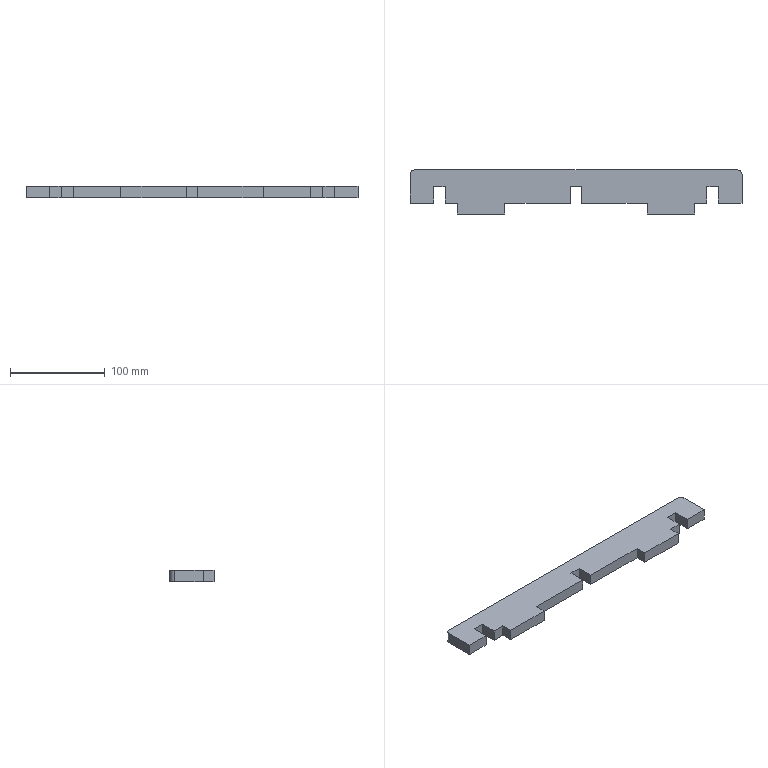Part | SolidWorks | features FlatPattern 1, SMBaseFlange 1, SheetMetal 1 | 1 solid | 28 faces | box 350 x 46.5 x 12 mm | volume 153111 mm3 | plane 26 | cylinder 2 | commonest cylinder face diameters 10 x2
STEP:
#1=CARTESIAN_POINT('',(187.743,-232.937,0.));
#2=VERTEX_POINT('',#1);
#3=CARTESIAN_POINT('',(187.743,-202.937,0.));
#4=VERTEX_POINT('',#3);
#5=CARTESIAN_POINT('',(187.743,-202.937,0.));
#6=DIRECTION('',(0.,1.,0.));
#7=VECTOR('',#6,1000.);
#8=LINE('',#5,#7);
#9=EDGE_CURVE('',#2,#4,#8,.T.);
#10=ORIENTED_EDGE('',*,*,#9,.F.);
#11=CARTESIAN_POINT('',(187.743,-232.937,-12.));
#12=VERTEX_POINT('',#11);
#13=CARTESIAN_POINT('',(187.743,-232.937,-12.));
#14=DIRECTION('',(0.,0.,1.));
#15=VECTOR('',#14,1000.);
#16=LINE('',#13,#15);
#17=EDGE_CURVE('',#12,#2,#16,.T.);
#18=ORIENTED_EDGE('',*,*,#17,.F.);
#19=CARTESIAN_POINT('',(187.743,-202.937,-12.));
#20=VERTEX_POINT('',#19);
#21=CARTESIAN_POINT('',(187.743,-202.937,-12.));
#22=DIRECTION('',(0.,1.,0.));
#23=VECTOR('',#22,1000.);
#24=LINE('',#21,#23);
#25=EDGE_CURVE('',#12,#20,#24,.T.);
#26=ORIENTED_EDGE('',*,*,#25,.T.);
#27=CARTESIAN_POINT('',(187.743,-202.937,-12.));
#28=DIRECTION('',(0.,0.,1.));
#29=VECTOR('',#28,1000.);
#30=LINE('',#27,#29);
#31=EDGE_CURVE('',#20,#4,#30,.T.);
#32=ORIENTED_EDGE('',*,*,#31,.T.);
#33=EDGE_LOOP('',(#10,#18,#26,#32));
#34=FACE_OUTER_BOUND('',#33,.T.);
#35=CARTESIAN_POINT('',(187.743,-202.937,-12.));
#36=DIRECTION('',(1.,0.,0.));
#37=DIRECTION('',(0.,0.,-1.));
#38=AXIS2_PLACEMENT_3D('',#35,#36,#37);
#39=PLANE('',#38);
#40=ADVANCED_FACE('',(#34),#39,.T.);
#41=CARTESIAN_POINT('',(162.743,-232.937,0.));
#42=VERTEX_POINT('',#41);
#43=CARTESIAN_POINT('',(187.743,-232.937,0.));
#44=DIRECTION('',(1.,0.,0.));
#45=VECTOR('',#44,1000.);
#46=LINE('',#43,#45);
#47=EDGE_CURVE('',#42,#2,#46,.T.);
#48=ORIENTED_EDGE('',*,*,#47,.F.);
#49=CARTESIAN_POINT('',(162.743,-232.937,-12.));
#50=VERTEX_POINT('',#49);
#51=CARTESIAN_POINT('',(162.743,-232.937,-12.));
#52=DIRECTION('',(0.,0.,1.));
#53=VECTOR('',#52,1000.);
#54=LINE('',#51,#53);
#55=EDGE_CURVE('',#50,#42,#54,.T.);
#56=ORIENTED_EDGE('',*,*,#55,.F.);
#57=CARTESIAN_POINT('',(187.743,-232.937,-12.));
#58=DIRECTION('',(1.,0.,0.));
#59=VECTOR('',#58,1000.);
#60=LINE('',#57,#59);
#61=EDGE_CURVE('',#50,#12,#60,.T.);
#62=ORIENTED_EDGE('',*,*,#61,.T.);
#63=ORIENTED_EDGE('',*,*,#17,.T.);
#64=EDGE_LOOP('',(#48,#56,#62,#63));
#65=FACE_OUTER_BOUND('',#64,.T.);
#66=CARTESIAN_POINT('',(187.743,-232.937,-12.));
#67=DIRECTION('',(0.,-1.,0.));
#68=DIRECTION('',(0.,0.,-1.));
#69=AXIS2_PLACEMENT_3D('',#66,#67,#68);
#70=PLANE('',#69);
#71=ADVANCED_FACE('',(#65),#70,.T.);
#72=CARTESIAN_POINT('',(162.743,-215.437,0.));
#73=VERTEX_POINT('',#72);
#74=CARTESIAN_POINT('',(162.743,-232.937,0.));
#75=DIRECTION('',(0.,-1.,0.));
#76=VECTOR('',#75,1000.);
#77=LINE('',#74,#76);
#78=EDGE_CURVE('',#73,#42,#77,.T.);
#79=ORIENTED_EDGE('',*,*,#78,.F.);
#80=CARTESIAN_POINT('',(162.743,-215.437,-12.));
#81=VERTEX_POINT('',#80);
#82=CARTESIAN_POINT('',(162.743,-215.437,-12.));
#83=DIRECTION('',(0.,0.,1.));
#84=VECTOR('',#83,1000.);
#85=LINE('',#82,#84);
#86=EDGE_CURVE('',#81,#73,#85,.T.);
#87=ORIENTED_EDGE('',*,*,#86,.F.);
#88=CARTESIAN_POINT('',(162.743,-232.937,-12.));
#89=DIRECTION('',(0.,-1.,0.));
#90=VECTOR('',#89,1000.);
#91=LINE('',#88,#90);
#92=EDGE_CURVE('',#81,#50,#91,.T.);
#93=ORIENTED_EDGE('',*,*,#92,.T.);
#94=ORIENTED_EDGE('',*,*,#55,.T.);
#95=EDGE_LOOP('',(#79,#87,#93,#94));
#96=FACE_OUTER_BOUND('',#95,.T.);
#97=CARTESIAN_POINT('',(162.743,-232.937,-12.));
#98=DIRECTION('',(-1.,0.,0.));
#99=DIRECTION('',(0.,-1.,0.));
#100=AXIS2_PLACEMENT_3D('',#97,#98,#99);
#101=PLANE('',#100);
#102=ADVANCED_FACE('',(#96),#101,.T.);
#103=CARTESIAN_POINT('',(150.743,-215.437,0.));
#104=VERTEX_POINT('',#103);
#105=CARTESIAN_POINT('',(162.743,-215.437,0.));
#106=DIRECTION('',(1.,0.,0.));
#107=VECTOR('',#106,1000.);
#108=LINE('',#105,#107);
#109=EDGE_CURVE('',#104,#73,#108,.T.);
#110=ORIENTED_EDGE('',*,*,#109,.F.);
#111=CARTESIAN_POINT('',(150.743,-215.437,-12.));
#112=VERTEX_POINT('',#111);
#113=CARTESIAN_POINT('',(150.743,-215.437,-12.));
#114=DIRECTION('',(0.,0.,1.));
#115=VECTOR('',#114,1000.);
#116=LINE('',#113,#115);
#117=EDGE_CURVE('',#112,#104,#116,.T.);
#118=ORIENTED_EDGE('',*,*,#117,.F.);
#119=CARTESIAN_POINT('',(162.743,-215.437,-12.));
#120=DIRECTION('',(1.,0.,0.));
#121=VECTOR('',#120,1000.);
#122=LINE('',#119,#121);
#123=EDGE_CURVE('',#112,#81,#122,.T.);
#124=ORIENTED_EDGE('',*,*,#123,.T.);
#125=ORIENTED_EDGE('',*,*,#86,.T.);
#126=EDGE_LOOP('',(#110,#118,#124,#125));
#127=FACE_OUTER_BOUND('',#126,.T.);
#128=CARTESIAN_POINT('',(162.743,-215.437,-12.));
#129=DIRECTION('',(0.,-1.,0.));
#130=DIRECTION('',(0.,0.,-1.));
#131=AXIS2_PLACEMENT_3D('',#128,#129,#130);
#132=PLANE('',#131);
#133=ADVANCED_FACE('',(#127),#132,.T.);
#134=CARTESIAN_POINT('',(150.743,-232.937,0.));
#135=VERTEX_POINT('',#134);
#136=CARTESIAN_POINT('',(150.743,-215.437,0.));
#137=DIRECTION('',(0.,1.,0.));
#138=VECTOR('',#137,1000.);
#139=LINE('',#136,#138);
#140=EDGE_CURVE('',#135,#104,#139,.T.);
#141=ORIENTED_EDGE('',*,*,#140,.F.);
#142=CARTESIAN_POINT('',(150.743,-232.937,-12.));
#143=VERTEX_POINT('',#142);
#144=CARTESIAN_POINT('',(150.743,-232.937,-12.));
#145=DIRECTION('',(0.,0.,1.));
#146=VECTOR('',#145,1000.);
#147=LINE('',#144,#146);
#148=EDGE_CURVE('',#143,#135,#147,.T.);
#149=ORIENTED_EDGE('',*,*,#148,.F.);
#150=CARTESIAN_POINT('',(150.743,-215.437,-12.));
#151=DIRECTION('',(0.,1.,0.));
#152=VECTOR('',#151,1000.);
#153=LINE('',#150,#152);
#154=EDGE_CURVE('',#143,#112,#153,.T.);
#155=ORIENTED_EDGE('',*,*,#154,.T.);
#156=ORIENTED_EDGE('',*,*,#117,.T.);
#157=EDGE_LOOP('',(#141,#149,#155,#156));
#158=FACE_OUTER_BOUND('',#157,.T.);
#159=CARTESIAN_POINT('',(150.743,-215.437,-12.));
#160=DIRECTION('',(1.,0.,0.));
#161=DIRECTION('',(0.,0.,-1.));
#162=AXIS2_PLACEMENT_3D('',#159,#160,#161);
#163=PLANE('',#162);
#164=ADVANCED_FACE('',(#158),#163,.T.);
#165=CARTESIAN_POINT('',(137.743,-232.937,0.));
#166=VERTEX_POINT('',#165);
#167=CARTESIAN_POINT('',(150.743,-232.937,0.));
#168=DIRECTION('',(1.,0.,0.));
#169=VECTOR('',#168,1000.);
#170=LINE('',#167,#169);
#171=EDGE_CURVE('',#166,#135,#170,.T.);
#172=ORIENTED_EDGE('',*,*,#171,.F.);
#173=CARTESIAN_POINT('',(137.743,-232.937,-12.));
#174=VERTEX_POINT('',#173);
#175=CARTESIAN_POINT('',(137.743,-232.937,-12.));
#176=DIRECTION('',(0.,0.,1.));
#177=VECTOR('',#176,1000.);
#178=LINE('',#175,#177);
#179=EDGE_CURVE('',#174,#166,#178,.T.);
#180=ORIENTED_EDGE('',*,*,#179,.F.);
#181=CARTESIAN_POINT('',(150.743,-232.937,-12.));
#182=DIRECTION('',(1.,0.,0.));
#183=VECTOR('',#182,1000.);
#184=LINE('',#181,#183);
#185=EDGE_CURVE('',#174,#143,#184,.T.);
#186=ORIENTED_EDGE('',*,*,#185,.T.);
#187=ORIENTED_EDGE('',*,*,#148,.T.);
#188=EDGE_LOOP('',(#172,#180,#186,#187));
#189=FACE_OUTER_BOUND('',#188,.T.);
#190=CARTESIAN_POINT('',(150.743,-232.937,-12.));
#191=DIRECTION('',(0.,-1.,0.));
#192=DIRECTION('',(0.,0.,-1.));
#193=AXIS2_PLACEMENT_3D('',#190,#191,#192);
#194=PLANE('',#193);
#195=ADVANCED_FACE('',(#189),#194,.T.);
#196=CARTESIAN_POINT('',(137.743,-244.437,0.));
#197=VERTEX_POINT('',#196);
#198=CARTESIAN_POINT('',(137.743,-232.937,0.));
#199=DIRECTION('',(0.,1.,0.));
#200=VECTOR('',#199,1000.);
#201=LINE('',#198,#200);
#202=EDGE_CURVE('',#197,#166,#201,.T.);
#203=ORIENTED_EDGE('',*,*,#202,.F.);
#204=CARTESIAN_POINT('',(137.743,-244.437,-12.));
#205=VERTEX_POINT('',#204);
#206=CARTESIAN_POINT('',(137.743,-244.437,-12.));
#207=DIRECTION('',(0.,0.,1.));
#208=VECTOR('',#207,1000.);
#209=LINE('',#206,#208);
#210=EDGE_CURVE('',#205,#197,#209,.T.);
#211=ORIENTED_EDGE('',*,*,#210,.F.);
#212=CARTESIAN_POINT('',(137.743,-232.937,-12.));
#213=DIRECTION('',(0.,1.,0.));
#214=VECTOR('',#213,1000.);
#215=LINE('',#212,#214);
#216=EDGE_CURVE('',#205,#174,#215,.T.);
#217=ORIENTED_EDGE('',*,*,#216,.T.);
#218=ORIENTED_EDGE('',*,*,#179,.T.);
#219=EDGE_LOOP('',(#203,#211,#217,#218));
#220=FACE_OUTER_BOUND('',#219,.T.);
#221=CARTESIAN_POINT('',(137.743,-232.937,-12.));
#222=DIRECTION('',(1.,0.,0.));
#223=DIRECTION('',(0.,0.,-1.));
#224=AXIS2_PLACEMENT_3D('',#221,#222,#223);
#225=PLANE('',#224);
#226=ADVANCED_FACE('',(#220),#225,.T.);
#227=CARTESIAN_POINT('',(87.743,-244.437,0.));
#228=VERTEX_POINT('',#227);
#229=CARTESIAN_POINT('',(137.743,-244.437,0.));
#230=DIRECTION('',(1.,0.,0.));
#231=VECTOR('',#230,1000.);
#232=LINE('',#229,#231);
#233=EDGE_CURVE('',#228,#197,#232,.T.);
#234=ORIENTED_EDGE('',*,*,#233,.F.);
#235=CARTESIAN_POINT('',(87.743,-244.437,-12.));
#236=VERTEX_POINT('',#235);
#237=CARTESIAN_POINT('',(87.743,-244.437,-12.));
#238=DIRECTION('',(0.,0.,1.));
#239=VECTOR('',#238,1000.);
#240=LINE('',#237,#239);
#241=EDGE_CURVE('',#236,#228,#240,.T.);
#242=ORIENTED_EDGE('',*,*,#241,.F.);
#243=CARTESIAN_POINT('',(137.743,-244.437,-12.));
#244=DIRECTION('',(1.,0.,0.));
#245=VECTOR('',#244,1000.);
#246=LINE('',#243,#245);
#247=EDGE_CURVE('',#236,#205,#246,.T.);
#248=ORIENTED_EDGE('',*,*,#247,.T.);
#249=ORIENTED_EDGE('',*,*,#210,.T.);
#250=EDGE_LOOP('',(#234,#242,#248,#249));
#251=FACE_OUTER_BOUND('',#250,.T.);
#252=CARTESIAN_POINT('',(137.743,-244.437,-12.));
#253=DIRECTION('',(0.,-1.,0.));
#254=DIRECTION('',(0.,0.,-1.));
#255=AXIS2_PLACEMENT_3D('',#252,#253,#254);
#256=PLANE('',#255);
#257=ADVANCED_FACE('',(#251),#256,.T.);
#258=CARTESIAN_POINT('',(87.743,-232.937,0.));
#259=VERTEX_POINT('',#258);
#260=CARTESIAN_POINT('',(87.743,-244.437,0.));
#261=DIRECTION('',(0.,-1.,0.));
#262=VECTOR('',#261,1000.);
#263=LINE('',#260,#262);
#264=EDGE_CURVE('',#259,#228,#263,.T.);
#265=ORIENTED_EDGE('',*,*,#264,.F.);
#266=CARTESIAN_POINT('',(87.743,-232.937,-12.));
#267=VERTEX_POINT('',#266);
#268=CARTESIAN_POINT('',(87.743,-232.937,-12.));
#269=DIRECTION('',(0.,0.,1.));
#270=VECTOR('',#269,1000.);
#271=LINE('',#268,#270);
#272=EDGE_CURVE('',#267,#259,#271,.T.);
#273=ORIENTED_EDGE('',*,*,#272,.F.);
#274=CARTESIAN_POINT('',(87.743,-244.437,-12.));
#275=DIRECTION('',(0.,-1.,0.));
#276=VECTOR('',#275,1000.);
#277=LINE('',#274,#276);
#278=EDGE_CURVE('',#267,#236,#277,.T.);
#279=ORIENTED_EDGE('',*,*,#278,.T.);
#280=ORIENTED_EDGE('',*,*,#241,.T.);
#281=EDGE_LOOP('',(#265,#273,#279,#280));
#282=FACE_OUTER_BOUND('',#281,.T.);
#283=CARTESIAN_POINT('',(87.743,-244.437,-12.));
#284=DIRECTION('',(-1.,0.,0.));
#285=DIRECTION('',(0.,0.,1.));
#286=AXIS2_PLACEMENT_3D('',#283,#284,#285);
#287=PLANE('',#286);
#288=ADVANCED_FACE('',(#282),#287,.T.);
#289=CARTESIAN_POINT('',(18.743,-232.937,0.));
#290=VERTEX_POINT('',#289);
#291=CARTESIAN_POINT('',(87.743,-232.937,0.));
#292=DIRECTION('',(1.,0.,0.));
#293=VECTOR('',#292,1000.);
#294=LINE('',#291,#293);
#295=EDGE_CURVE('',#290,#259,#294,.T.);
#296=ORIENTED_EDGE('',*,*,#295,.F.);
#297=CARTESIAN_POINT('',(18.743,-232.937,-12.));
#298=VERTEX_POINT('',#297);
#299=CARTESIAN_POINT('',(18.743,-232.937,-12.));
#300=DIRECTION('',(0.,0.,1.));
#301=VECTOR('',#300,1000.);
#302=LINE('',#299,#301);
#303=EDGE_CURVE('',#298,#290,#302,.T.);
#304=ORIENTED_EDGE('',*,*,#303,.F.);
#305=CARTESIAN_POINT('',(87.743,-232.937,-12.));
#306=DIRECTION('',(1.,0.,0.));
#307=VECTOR('',#306,1000.);
#308=LINE('',#305,#307);
#309=EDGE_CURVE('',#298,#267,#308,.T.);
#310=ORIENTED_EDGE('',*,*,#309,.T.);
#311=ORIENTED_EDGE('',*,*,#272,.T.);
#312=EDGE_LOOP('',(#296,#304,#310,#311));
#313=FACE_OUTER_BOUND('',#312,.T.);
#314=CARTESIAN_POINT('',(87.743,-232.937,-12.));
#315=DIRECTION('',(0.,-1.,0.));
#316=DIRECTION('',(1.,0.,0.));
#317=AXIS2_PLACEMENT_3D('',#314,#315,#316);
#318=PLANE('',#317);
#319=ADVANCED_FACE('',(#313),#318,.T.);
#320=CARTESIAN_POINT('',(18.743,-215.437,0.));
#321=VERTEX_POINT('',#320);
#322=CARTESIAN_POINT('',(18.743,-232.937,0.));
#323=DIRECTION('',(0.,-1.,0.));
#324=VECTOR('',#323,1000.);
#325=LINE('',#322,#324);
#326=EDGE_CURVE('',#321,#290,#325,.T.);
#327=ORIENTED_EDGE('',*,*,#326,.F.);
#328=CARTESIAN_POINT('',(18.743,-215.437,-12.));
#329=VERTEX_POINT('',#328);
#330=CARTESIAN_POINT('',(18.743,-215.437,-12.));
#331=DIRECTION('',(0.,0.,1.));
#332=VECTOR('',#331,1000.);
#333=LINE('',#330,#332);
#334=EDGE_CURVE('',#329,#321,#333,.T.);
#335=ORIENTED_EDGE('',*,*,#334,.F.);
#336=CARTESIAN_POINT('',(18.743,-232.937,-12.));
#337=DIRECTION('',(0.,-1.,0.));
#338=VECTOR('',#337,1000.);
#339=LINE('',#336,#338);
#340=EDGE_CURVE('',#329,#298,#339,.T.);
#341=ORIENTED_EDGE('',*,*,#340,.T.);
#342=ORIENTED_EDGE('',*,*,#303,.T.);
#343=EDGE_LOOP('',(#327,#335,#341,#342));
#344=FACE_OUTER_BOUND('',#343,.T.);
#345=CARTESIAN_POINT('',(18.743,-232.937,-12.));
#346=DIRECTION('',(-1.,0.,0.));
#347=DIRECTION('',(0.,0.,1.));
#348=AXIS2_PLACEMENT_3D('',#345,#346,#347);
#349=PLANE('',#348);
#350=ADVANCED_FACE('',(#344),#349,.T.);
#351=CARTESIAN_POINT('',(6.743,-215.437,0.));
#352=VERTEX_POINT('',#351);
#353=CARTESIAN_POINT('',(18.743,-215.437,0.));
#354=DIRECTION('',(1.,0.,0.));
#355=VECTOR('',#354,1000.);
#356=LINE('',#353,#355);
#357=EDGE_CURVE('',#352,#321,#356,.T.);
#358=ORIENTED_EDGE('',*,*,#357,.F.);
#359=CARTESIAN_POINT('',(6.743,-215.437,-12.));
#360=VERTEX_POINT('',#359);
#361=CARTESIAN_POINT('',(6.743,-215.437,-12.));
#362=DIRECTION('',(0.,0.,1.));
#363=VECTOR('',#362,1000.);
#364=LINE('',#361,#363);
#365=EDGE_CURVE('',#360,#352,#364,.T.);
#366=ORIENTED_EDGE('',*,*,#365,.F.);
#367=CARTESIAN_POINT('',(18.743,-215.437,-12.));
#368=DIRECTION('',(1.,0.,0.));
#369=VECTOR('',#368,1000.);
#370=LINE('',#367,#369);
#371=EDGE_CURVE('',#360,#329,#370,.T.);
#372=ORIENTED_EDGE('',*,*,#371,.T.);
#373=ORIENTED_EDGE('',*,*,#334,.T.);
#374=EDGE_LOOP('',(#358,#366,#372,#373));
#375=FACE_OUTER_BOUND('',#374,.T.);
#376=CARTESIAN_POINT('',(18.743,-215.437,-12.));
#377=DIRECTION('',(0.,-1.,0.));
#378=DIRECTION('',(0.,0.,-1.));
#379=AXIS2_PLACEMENT_3D('',#376,#377,#378);
#380=PLANE('',#379);
#381=ADVANCED_FACE('',(#375),#380,.T.);
#382=CARTESIAN_POINT('',(6.743,-232.937,0.));
#383=VERTEX_POINT('',#382);
#384=CARTESIAN_POINT('',(6.743,-215.437,0.));
#385=DIRECTION('',(0.,1.,0.));
#386=VECTOR('',#385,1000.);
#387=LINE('',#384,#386);
#388=EDGE_CURVE('',#383,#352,#387,.T.);
#389=ORIENTED_EDGE('',*,*,#388,.F.);
#390=CARTESIAN_POINT('',(6.743,-232.937,-12.));
#391=VERTEX_POINT('',#390);
#392=CARTESIAN_POINT('',(6.743,-232.937,-12.));
#393=DIRECTION('',(0.,0.,1.));
#394=VECTOR('',#393,1000.);
#395=LINE('',#392,#394);
#396=EDGE_CURVE('',#391,#383,#395,.T.);
#397=ORIENTED_EDGE('',*,*,#396,.F.);
#398=CARTESIAN_POINT('',(6.743,-215.437,-12.));
#399=DIRECTION('',(0.,1.,0.));
#400=VECTOR('',#399,1000.);
#401=LINE('',#398,#400);
#402=EDGE_CURVE('',#391,#360,#401,.T.);
#403=ORIENTED_EDGE('',*,*,#402,.T.);
#404=ORIENTED_EDGE('',*,*,#365,.T.);
#405=EDGE_LOOP('',(#389,#397,#403,#404));
#406=FACE_OUTER_BOUND('',#405,.T.);
#407=CARTESIAN_POINT('',(6.743,-215.437,-12.));
#408=DIRECTION('',(1.,0.,0.));
#409=DIRECTION('',(0.,0.,-1.));
#410=AXIS2_PLACEMENT_3D('',#407,#408,#409);
#411=PLANE('',#410);
#412=ADVANCED_FACE('',(#406),#411,.T.);
#413=CARTESIAN_POINT('',(-62.257,-232.937,0.));
#414=VERTEX_POINT('',#413);
#415=CARTESIAN_POINT('',(6.743,-232.937,0.));
#416=DIRECTION('',(1.,0.,0.));
#417=VECTOR('',#416,1000.);
#418=LINE('',#415,#417);
#419=EDGE_CURVE('',#414,#383,#418,.T.);
#420=ORIENTED_EDGE('',*,*,#419,.F.);
#421=CARTESIAN_POINT('',(-62.257,-232.937,-12.));
#422=VERTEX_POINT('',#421);
#423=CARTESIAN_POINT('',(-62.257,-232.937,-12.));
#424=DIRECTION('',(0.,0.,1.));
#425=VECTOR('',#424,1000.);
#426=LINE('',#423,#425);
#427=EDGE_CURVE('',#422,#414,#426,.T.);
#428=ORIENTED_EDGE('',*,*,#427,.F.);
#429=CARTESIAN_POINT('',(6.743,-232.937,-12.));
#430=DIRECTION('',(1.,0.,0.));
#431=VECTOR('',#430,1000.);
#432=LINE('',#429,#431);
#433=EDGE_CURVE('',#422,#391,#432,.T.);
#434=ORIENTED_EDGE('',*,*,#433,.T.);
#435=ORIENTED_EDGE('',*,*,#396,.T.);
#436=EDGE_LOOP('',(#420,#428,#434,#435));
#437=FACE_OUTER_BOUND('',#436,.T.);
#438=CARTESIAN_POINT('',(6.743,-232.937,-12.));
#439=DIRECTION('',(0.,-1.,0.));
#440=DIRECTION('',(1.,0.,0.));
#441=AXIS2_PLACEMENT_3D('',#438,#439,#440);
#442=PLANE('',#441);
#443=ADVANCED_FACE('',(#437),#442,.T.);
#444=CARTESIAN_POINT('',(-62.257,-244.437,0.));
#445=VERTEX_POINT('',#444);
#446=CARTESIAN_POINT('',(-62.257,-232.937,0.));
#447=DIRECTION('',(0.,1.,0.));
#448=VECTOR('',#447,1000.);
#449=LINE('',#446,#448);
#450=EDGE_CURVE('',#445,#414,#449,.T.);
#451=ORIENTED_EDGE('',*,*,#450,.F.);
#452=CARTESIAN_POINT('',(-62.257,-244.437,-12.));
#453=VERTEX_POINT('',#452);
#454=CARTESIAN_POINT('',(-62.257,-244.437,-12.));
#455=DIRECTION('',(0.,0.,1.));
#456=VECTOR('',#455,1000.);
#457=LINE('',#454,#456);
#458=EDGE_CURVE('',#453,#445,#457,.T.);
#459=ORIENTED_EDGE('',*,*,#458,.F.);
#460=CARTESIAN_POINT('',(-62.257,-232.937,-12.));
#461=DIRECTION('',(0.,1.,0.));
#462=VECTOR('',#461,1000.);
#463=LINE('',#460,#462);
#464=EDGE_CURVE('',#453,#422,#463,.T.);
#465=ORIENTED_EDGE('',*,*,#464,.T.);
#466=ORIENTED_EDGE('',*,*,#427,.T.);
#467=EDGE_LOOP('',(#451,#459,#465,#466));
#468=FACE_OUTER_BOUND('',#467,.T.);
#469=CARTESIAN_POINT('',(-62.257,-232.937,-12.));
#470=DIRECTION('',(1.,0.,0.));
#471=DIRECTION('',(0.,0.,-1.));
#472=AXIS2_PLACEMENT_3D('',#469,#470,#471);
#473=PLANE('',#472);
#474=ADVANCED_FACE('',(#468),#473,.T.);
#475=CARTESIAN_POINT('',(-112.257,-244.437,0.));
#476=VERTEX_POINT('',#475);
#477=CARTESIAN_POINT('',(-62.257,-244.437,0.));
#478=DIRECTION('',(1.,0.,0.));
#479=VECTOR('',#478,1000.);
#480=LINE('',#477,#479);
#481=EDGE_CURVE('',#476,#445,#480,.T.);
#482=ORIENTED_EDGE('',*,*,#481,.F.);
#483=CARTESIAN_POINT('',(-112.257,-244.437,-12.));
#484=VERTEX_POINT('',#483);
#485=CARTESIAN_POINT('',(-112.257,-244.437,-12.));
#486=DIRECTION('',(0.,0.,1.));
#487=VECTOR('',#486,1000.);
#488=LINE('',#485,#487);
#489=EDGE_CURVE('',#484,#476,#488,.T.);
#490=ORIENTED_EDGE('',*,*,#489,.F.);
#491=CARTESIAN_POINT('',(-62.257,-244.437,-12.));
#492=DIRECTION('',(1.,0.,0.));
#493=VECTOR('',#492,1000.);
#494=LINE('',#491,#493);
#495=EDGE_CURVE('',#484,#453,#494,.T.);
#496=ORIENTED_EDGE('',*,*,#495,.T.);
#497=ORIENTED_EDGE('',*,*,#458,.T.);
#498=EDGE_LOOP('',(#482,#490,#496,#497));
#499=FACE_OUTER_BOUND('',#498,.T.);
#500=CARTESIAN_POINT('',(-62.257,-244.437,-12.));
#501=DIRECTION('',(0.,-1.,0.));
#502=DIRECTION('',(0.,0.,-1.));
#503=AXIS2_PLACEMENT_3D('',#500,#501,#502);
#504=PLANE('',#503);
#505=ADVANCED_FACE('',(#499),#504,.T.);
#506=CARTESIAN_POINT('',(-112.257,-232.937,0.));
#507=VERTEX_POINT('',#506);
#508=CARTESIAN_POINT('',(-112.257,-244.437,0.));
#509=DIRECTION('',(0.,-1.,0.));
#510=VECTOR('',#509,1000.);
#511=LINE('',#508,#510);
#512=EDGE_CURVE('',#507,#476,#511,.T.);
#513=ORIENTED_EDGE('',*,*,#512,.F.);
#514=CARTESIAN_POINT('',(-112.257,-232.937,-12.));
#515=VERTEX_POINT('',#514);
#516=CARTESIAN_POINT('',(-112.257,-232.937,-12.));
#517=DIRECTION('',(0.,0.,1.));
#518=VECTOR('',#517,1000.);
#519=LINE('',#516,#518);
#520=EDGE_CURVE('',#515,#507,#519,.T.);
#521=ORIENTED_EDGE('',*,*,#520,.F.);
#522=CARTESIAN_POINT('',(-112.257,-244.437,-12.));
#523=DIRECTION('',(0.,-1.,0.));
#524=VECTOR('',#523,1000.);
#525=LINE('',#522,#524);
#526=EDGE_CURVE('',#515,#484,#525,.T.);
#527=ORIENTED_EDGE('',*,*,#526,.T.);
#528=ORIENTED_EDGE('',*,*,#489,.T.);
#529=EDGE_LOOP('',(#513,#521,#527,#528));
#530=FACE_OUTER_BOUND('',#529,.T.);
#531=CARTESIAN_POINT('',(-112.257,-244.437,-12.));
#532=DIRECTION('',(-1.,0.,0.));
#533=DIRECTION('',(0.,0.,1.));
#534=AXIS2_PLACEMENT_3D('',#531,#532,#533);
#535=PLANE('',#534);
#536=ADVANCED_FACE('',(#530),#535,.T.);
#537=CARTESIAN_POINT('',(-125.257,-232.937,0.));
#538=VERTEX_POINT('',#537);
#539=CARTESIAN_POINT('',(-112.257,-232.937,0.));
#540=DIRECTION('',(1.,0.,0.));
#541=VECTOR('',#540,1000.);
#542=LINE('',#539,#541);
#543=EDGE_CURVE('',#538,#507,#542,.T.);
#544=ORIENTED_EDGE('',*,*,#543,.F.);
#545=CARTESIAN_POINT('',(-125.257,-232.937,-12.));
#546=VERTEX_POINT('',#545);
#547=CARTESIAN_POINT('',(-125.257,-232.937,-12.));
#548=DIRECTION('',(0.,0.,1.));
#549=VECTOR('',#548,1000.);
#550=LINE('',#547,#549);
#551=EDGE_CURVE('',#546,#538,#550,.T.);
#552=ORIENTED_EDGE('',*,*,#551,.F.);
#553=CARTESIAN_POINT('',(-112.257,-232.937,-12.));
#554=DIRECTION('',(1.,0.,0.));
#555=VECTOR('',#554,1000.);
#556=LINE('',#553,#555);
#557=EDGE_CURVE('',#546,#515,#556,.T.);
#558=ORIENTED_EDGE('',*,*,#557,.T.);
#559=ORIENTED_EDGE('',*,*,#520,.T.);
#560=EDGE_LOOP('',(#544,#552,#558,#559));
#561=FACE_OUTER_BOUND('',#560,.T.);
#562=CARTESIAN_POINT('',(-112.257,-232.937,-12.));
#563=DIRECTION('',(0.,-1.,0.));
#564=DIRECTION('',(1.,0.,0.));
#565=AXIS2_PLACEMENT_3D('',#562,#563,#564);
#566=PLANE('',#565);
#567=ADVANCED_FACE('',(#561),#566,.T.);
#568=CARTESIAN_POINT('',(-125.257,-215.437,0.));
#569=VERTEX_POINT('',#568);
#570=CARTESIAN_POINT('',(-125.257,-232.937,0.));
#571=DIRECTION('',(0.,-1.,0.));
#572=VECTOR('',#571,1000.);
#573=LINE('',#570,#572);
#574=EDGE_CURVE('',#569,#538,#573,.T.);
#575=ORIENTED_EDGE('',*,*,#574,.F.);
#576=CARTESIAN_POINT('',(-125.257,-215.437,-12.));
#577=VERTEX_POINT('',#576);
#578=CARTESIAN_POINT('',(-125.257,-215.437,-12.));
#579=DIRECTION('',(0.,0.,1.));
#580=VECTOR('',#579,1000.);
#581=LINE('',#578,#580);
#582=EDGE_CURVE('',#577,#569,#581,.T.);
#583=ORIENTED_EDGE('',*,*,#582,.F.);
#584=CARTESIAN_POINT('',(-125.257,-232.937,-12.));
#585=DIRECTION('',(0.,-1.,0.));
#586=VECTOR('',#585,1000.);
#587=LINE('',#584,#586);
#588=EDGE_CURVE('',#577,#546,#587,.T.);
#589=ORIENTED_EDGE('',*,*,#588,.T.);
#590=ORIENTED_EDGE('',*,*,#551,.T.);
#591=EDGE_LOOP('',(#575,#583,#589,#590));
#592=FACE_OUTER_BOUND('',#591,.T.);
#593=CARTESIAN_POINT('',(-125.257,-232.937,-12.));
#594=DIRECTION('',(-1.,0.,0.));
#595=DIRECTION('',(0.,0.,1.));
#596=AXIS2_PLACEMENT_3D('',#593,#594,#595);
#597=PLANE('',#596);
#598=ADVANCED_FACE('',(#592),#597,.T.);
#599=CARTESIAN_POINT('',(-137.257,-215.437,0.));
#600=VERTEX_POINT('',#599);
#601=CARTESIAN_POINT('',(-125.257,-215.437,0.));
#602=DIRECTION('',(1.,0.,0.));
#603=VECTOR('',#602,1000.);
#604=LINE('',#601,#603);
#605=EDGE_CURVE('',#600,#569,#604,.T.);
#606=ORIENTED_EDGE('',*,*,#605,.F.);
#607=CARTESIAN_POINT('',(-137.257,-215.437,-12.));
#608=VERTEX_POINT('',#607);
#609=CARTESIAN_POINT('',(-137.257,-215.437,-12.));
#610=DIRECTION('',(0.,0.,1.));
#611=VECTOR('',#610,1000.);
#612=LINE('',#609,#611);
#613=EDGE_CURVE('',#608,#600,#612,.T.);
#614=ORIENTED_EDGE('',*,*,#613,.F.);
#615=CARTESIAN_POINT('',(-125.257,-215.437,-12.));
#616=DIRECTION('',(1.,0.,0.));
#617=VECTOR('',#616,1000.);
#618=LINE('',#615,#617);
#619=EDGE_CURVE('',#608,#577,#618,.T.);
#620=ORIENTED_EDGE('',*,*,#619,.T.);
#621=ORIENTED_EDGE('',*,*,#582,.T.);
#622=EDGE_LOOP('',(#606,#614,#620,#621));
#623=FACE_OUTER_BOUND('',#622,.T.);
#624=CARTESIAN_POINT('',(-125.257,-215.437,-12.));
#625=DIRECTION('',(0.,-1.,0.));
#626=DIRECTION('',(1.,0.,0.));
#627=AXIS2_PLACEMENT_3D('',#624,#625,#626);
#628=PLANE('',#627);
#629=ADVANCED_FACE('',(#623),#628,.T.);
#630=CARTESIAN_POINT('',(-137.257,-232.937,0.));
#631=VERTEX_POINT('',#630);
#632=CARTESIAN_POINT('',(-137.257,-215.437,0.));
#633=DIRECTION('',(0.,1.,0.));
#634=VECTOR('',#633,1000.);
#635=LINE('',#632,#634);
#636=EDGE_CURVE('',#631,#600,#635,.T.);
#637=ORIENTED_EDGE('',*,*,#636,.F.);
#638=CARTESIAN_POINT('',(-137.257,-232.937,-12.));
#639=VERTEX_POINT('',#638);
#640=CARTESIAN_POINT('',(-137.257,-232.937,-12.));
#641=DIRECTION('',(0.,0.,1.));
#642=VECTOR('',#641,1000.);
#643=LINE('',#640,#642);
#644=EDGE_CURVE('',#639,#631,#643,.T.);
#645=ORIENTED_EDGE('',*,*,#644,.F.);
#646=CARTESIAN_POINT('',(-137.257,-215.437,-12.));
#647=DIRECTION('',(0.,1.,0.));
#648=VECTOR('',#647,1000.);
#649=LINE('',#646,#648);
#650=EDGE_CURVE('',#639,#608,#649,.T.);
#651=ORIENTED_EDGE('',*,*,#650,.T.);
#652=ORIENTED_EDGE('',*,*,#613,.T.);
#653=EDGE_LOOP('',(#637,#645,#651,#652));
#654=FACE_OUTER_BOUND('',#653,.T.);
#655=CARTESIAN_POINT('',(-137.257,-215.437,-12.));
#656=DIRECTION('',(1.,0.,0.));
#657=DIRECTION('',(0.,0.,-1.));
#658=AXIS2_PLACEMENT_3D('',#655,#656,#657);
#659=PLANE('',#658);
#660=ADVANCED_FACE('',(#654),#659,.T.);
#661=CARTESIAN_POINT('',(-162.257,-232.937,0.));
#662=VERTEX_POINT('',#661);
#663=CARTESIAN_POINT('',(-137.257,-232.937,0.));
#664=DIRECTION('',(1.,0.,0.));
#665=VECTOR('',#664,1000.);
#666=LINE('',#663,#665);
#667=EDGE_CURVE('',#662,#631,#666,.T.);
#668=ORIENTED_EDGE('',*,*,#667,.F.);
#669=CARTESIAN_POINT('',(-162.257,-232.937,-12.));
#670=VERTEX_POINT('',#669);
#671=CARTESIAN_POINT('',(-162.257,-232.937,-12.));
#672=DIRECTION('',(0.,0.,1.));
#673=VECTOR('',#672,1000.);
#674=LINE('',#671,#673);
#675=EDGE_CURVE('',#670,#662,#674,.T.);
#676=ORIENTED_EDGE('',*,*,#675,.F.);
#677=CARTESIAN_POINT('',(-137.257,-232.937,-12.));
#678=DIRECTION('',(1.,0.,0.));
#679=VECTOR('',#678,1000.);
#680=LINE('',#677,#679);
#681=EDGE_CURVE('',#670,#639,#680,.T.);
#682=ORIENTED_EDGE('',*,*,#681,.T.);
#683=ORIENTED_EDGE('',*,*,#644,.T.);
#684=EDGE_LOOP('',(#668,#676,#682,#683));
#685=FACE_OUTER_BOUND('',#684,.T.);
#686=CARTESIAN_POINT('',(-137.257,-232.937,-12.));
#687=DIRECTION('',(0.,-1.,0.));
#688=DIRECTION('',(1.,0.,0.));
#689=AXIS2_PLACEMENT_3D('',#686,#687,#688);
#690=PLANE('',#689);
#691=ADVANCED_FACE('',(#685),#690,.T.);
#692=CARTESIAN_POINT('',(-162.257,-202.937,0.));
#693=VERTEX_POINT('',#692);
#694=CARTESIAN_POINT('',(-162.257,-202.937,0.));
#695=DIRECTION('',(0.,-1.,0.));
#696=VECTOR('',#695,1000.);
#697=LINE('',#694,#696);
#698=EDGE_CURVE('',#693,#662,#697,.T.);
#699=ORIENTED_EDGE('',*,*,#698,.F.);
#700=CARTESIAN_POINT('',(-162.257,-202.937,-12.));
#701=VERTEX_POINT('',#700);
#702=CARTESIAN_POINT('',(-162.257,-202.937,-12.));
#703=DIRECTION('',(0.,0.,1.));
#704=VECTOR('',#703,1000.);
#705=LINE('',#702,#704);
#706=EDGE_CURVE('',#701,#693,#705,.T.);
#707=ORIENTED_EDGE('',*,*,#706,.F.);
#708=CARTESIAN_POINT('',(-162.257,-202.937,-12.));
#709=DIRECTION('',(0.,-1.,0.));
#710=VECTOR('',#709,1000.);
#711=LINE('',#708,#710);
#712=EDGE_CURVE('',#701,#670,#711,.T.);
#713=ORIENTED_EDGE('',*,*,#712,.T.);
#714=ORIENTED_EDGE('',*,*,#675,.T.);
#715=EDGE_LOOP('',(#699,#707,#713,#714));
#716=FACE_OUTER_BOUND('',#715,.T.);
#717=CARTESIAN_POINT('',(-162.257,-202.937,-12.));
#718=DIRECTION('',(-1.,0.,0.));
#719=DIRECTION('',(0.,-1.,0.));
#720=AXIS2_PLACEMENT_3D('',#717,#718,#719);
#721=PLANE('',#720);
#722=ADVANCED_FACE('',(#716),#721,.T.);
#723=CARTESIAN_POINT('',(-157.257,-197.937,0.));
#724=VERTEX_POINT('',#723);
#725=CARTESIAN_POINT('',(-157.257,-202.937,0.));
#726=DIRECTION('',(0.,0.,1.));
#727=DIRECTION('',(1.,0.,0.));
#728=AXIS2_PLACEMENT_3D('',#725,#726,#727);
#729=CIRCLE('',#728,5.);
#730=EDGE_CURVE('',#724,#693,#729,.T.);
#731=ORIENTED_EDGE('',*,*,#730,.F.);
#732=CARTESIAN_POINT('',(-157.257,-197.937,-12.));
#733=VERTEX_POINT('',#732);
#734=CARTESIAN_POINT('',(-157.257,-197.937,-12.));
#735=DIRECTION('',(0.,0.,1.));
#736=VECTOR('',#735,1000.);
#737=LINE('',#734,#736);
#738=EDGE_CURVE('',#733,#724,#737,.T.);
#739=ORIENTED_EDGE('',*,*,#738,.F.);
#740=CARTESIAN_POINT('',(-157.257,-202.937,-12.));
#741=DIRECTION('',(0.,0.,1.));
#742=DIRECTION('',(1.,0.,0.));
#743=AXIS2_PLACEMENT_3D('',#740,#741,#742);
#744=CIRCLE('',#743,5.);
#745=EDGE_CURVE('',#733,#701,#744,.T.);
#746=ORIENTED_EDGE('',*,*,#745,.T.);
#747=ORIENTED_EDGE('',*,*,#706,.T.);
#748=EDGE_LOOP('',(#731,#739,#746,#747));
#749=FACE_OUTER_BOUND('',#748,.T.);
#750=CARTESIAN_POINT('',(-157.257,-202.937,-12.));
#751=DIRECTION('',(0.,0.,1.));
#752=DIRECTION('',(1.,0.,0.));
#753=AXIS2_PLACEMENT_3D('',#750,#751,#752);
#754=CYLINDRICAL_SURFACE('',#753,5.);
#755=ADVANCED_FACE('',(#749),#754,.T.);
#756=CARTESIAN_POINT('',(182.743,-197.937,0.));
#757=VERTEX_POINT('',#756);
#758=CARTESIAN_POINT('',(182.743,-197.937,0.));
#759=DIRECTION('',(-1.,0.,0.));
#760=VECTOR('',#759,1000.);
#761=LINE('',#758,#760);
#762=EDGE_CURVE('',#757,#724,#761,.T.);
#763=ORIENTED_EDGE('',*,*,#762,.F.);
#764=CARTESIAN_POINT('',(182.743,-197.937,-12.));
#765=VERTEX_POINT('',#764);
#766=CARTESIAN_POINT('',(182.743,-197.937,-12.));
#767=DIRECTION('',(0.,0.,1.));
#768=VECTOR('',#767,1000.);
#769=LINE('',#766,#768);
#770=EDGE_CURVE('',#765,#757,#769,.T.);
#771=ORIENTED_EDGE('',*,*,#770,.F.);
#772=CARTESIAN_POINT('',(182.743,-197.937,-12.));
#773=DIRECTION('',(-1.,0.,0.));
#774=VECTOR('',#773,1000.);
#775=LINE('',#772,#774);
#776=EDGE_CURVE('',#765,#733,#775,.T.);
#777=ORIENTED_EDGE('',*,*,#776,.T.);
#778=ORIENTED_EDGE('',*,*,#738,.T.);
#779=EDGE_LOOP('',(#763,#771,#777,#778));
#780=FACE_OUTER_BOUND('',#779,.T.);
#781=CARTESIAN_POINT('',(182.743,-197.937,-12.));
#782=DIRECTION('',(0.,1.,0.));
#783=DIRECTION('',(0.,0.,1.));
#784=AXIS2_PLACEMENT_3D('',#781,#782,#783);
#785=PLANE('',#784);
#786=ADVANCED_FACE('',(#780),#785,.T.);
#787=CARTESIAN_POINT('',(182.743,-202.937,0.));
#788=DIRECTION('',(0.,0.,1.));
#789=DIRECTION('',(1.,0.,0.));
#790=AXIS2_PLACEMENT_3D('',#787,#788,#789);
#791=CIRCLE('',#790,5.);
#792=EDGE_CURVE('',#4,#757,#791,.T.);
#793=ORIENTED_EDGE('',*,*,#792,.F.);
#794=ORIENTED_EDGE('',*,*,#31,.F.);
#795=CARTESIAN_POINT('',(182.743,-202.937,-12.));
#796=DIRECTION('',(0.,0.,1.));
#797=DIRECTION('',(1.,0.,0.));
#798=AXIS2_PLACEMENT_3D('',#795,#796,#797);
#799=CIRCLE('',#798,5.);
#800=EDGE_CURVE('',#20,#765,#799,.T.);
#801=ORIENTED_EDGE('',*,*,#800,.T.);
#802=ORIENTED_EDGE('',*,*,#770,.T.);
#803=EDGE_LOOP('',(#793,#794,#801,#802));
#804=FACE_OUTER_BOUND('',#803,.T.);
#805=CARTESIAN_POINT('',(182.743,-202.937,-12.));
#806=DIRECTION('',(0.,0.,1.));
#807=DIRECTION('',(1.,0.,0.));
#808=AXIS2_PLACEMENT_3D('',#805,#806,#807);
#809=CYLINDRICAL_SURFACE('',#808,5.);
#810=ADVANCED_FACE('',(#804),#809,.T.);
#811=ORIENTED_EDGE('',*,*,#25,.F.);
#812=ORIENTED_EDGE('',*,*,#61,.F.);
#813=ORIENTED_EDGE('',*,*,#92,.F.);
#814=ORIENTED_EDGE('',*,*,#123,.F.);
#815=ORIENTED_EDGE('',*,*,#154,.F.);
#816=ORIENTED_EDGE('',*,*,#185,.F.);
#817=ORIENTED_EDGE('',*,*,#216,.F.);
#818=ORIENTED_EDGE('',*,*,#247,.F.);
#819=ORIENTED_EDGE('',*,*,#278,.F.);
#820=ORIENTED_EDGE('',*,*,#309,.F.);
#821=ORIENTED_EDGE('',*,*,#340,.F.);
#822=ORIENTED_EDGE('',*,*,#371,.F.);
#823=ORIENTED_EDGE('',*,*,#402,.F.);
#824=ORIENTED_EDGE('',*,*,#433,.F.);
#825=ORIENTED_EDGE('',*,*,#464,.F.);
#826=ORIENTED_EDGE('',*,*,#495,.F.);
#827=ORIENTED_EDGE('',*,*,#526,.F.);
#828=ORIENTED_EDGE('',*,*,#557,.F.);
#829=ORIENTED_EDGE('',*,*,#588,.F.);
#830=ORIENTED_EDGE('',*,*,#619,.F.);
#831=ORIENTED_EDGE('',*,*,#650,.F.);
#832=ORIENTED_EDGE('',*,*,#681,.F.);
#833=ORIENTED_EDGE('',*,*,#712,.F.);
#834=ORIENTED_EDGE('',*,*,#745,.F.);
#835=ORIENTED_EDGE('',*,*,#776,.F.);
#836=ORIENTED_EDGE('',*,*,#800,.F.);
#837=EDGE_LOOP('',(#811,#812,#813,#814,#815,#816,#817,#818,#819,#820,#821,#822,#823,#824,#825,#826,#827,#828,#829,#830,#831,#832,#833,#834,#835,#836));
#838=FACE_OUTER_BOUND('',#837,.T.);
#839=CARTESIAN_POINT('',(-157.257,-202.937,-12.));
#840=DIRECTION('',(0.,0.,1.));
#841=DIRECTION('',(1.,0.,0.));
#842=AXIS2_PLACEMENT_3D('',#839,#840,#841);
#843=PLANE('',#842);
#844=ADVANCED_FACE('',(#838),#843,.F.);
#845=ORIENTED_EDGE('',*,*,#9,.T.);
#846=ORIENTED_EDGE('',*,*,#792,.T.);
#847=ORIENTED_EDGE('',*,*,#762,.T.);
#848=ORIENTED_EDGE('',*,*,#730,.T.);
#849=ORIENTED_EDGE('',*,*,#698,.T.);
#850=ORIENTED_EDGE('',*,*,#667,.T.);
#851=ORIENTED_EDGE('',*,*,#636,.T.);
#852=ORIENTED_EDGE('',*,*,#605,.T.);
#853=ORIENTED_EDGE('',*,*,#574,.T.);
#854=ORIENTED_EDGE('',*,*,#543,.T.);
#855=ORIENTED_EDGE('',*,*,#512,.T.);
#856=ORIENTED_EDGE('',*,*,#481,.T.);
#857=ORIENTED_EDGE('',*,*,#450,.T.);
#858=ORIENTED_EDGE('',*,*,#419,.T.);
#859=ORIENTED_EDGE('',*,*,#388,.T.);
#860=ORIENTED_EDGE('',*,*,#357,.T.);
#861=ORIENTED_EDGE('',*,*,#326,.T.);
#862=ORIENTED_EDGE('',*,*,#295,.T.);
#863=ORIENTED_EDGE('',*,*,#264,.T.);
#864=ORIENTED_EDGE('',*,*,#233,.T.);
#865=ORIENTED_EDGE('',*,*,#202,.T.);
#866=ORIENTED_EDGE('',*,*,#171,.T.);
#867=ORIENTED_EDGE('',*,*,#140,.T.);
#868=ORIENTED_EDGE('',*,*,#109,.T.);
#869=ORIENTED_EDGE('',*,*,#78,.T.);
#870=ORIENTED_EDGE('',*,*,#47,.T.);
#871=EDGE_LOOP('',(#845,#846,#847,#848,#849,#850,#851,#852,#853,#854,#855,#856,#857,#858,#859,#860,#861,#862,#863,#864,#865,#866,#867,#868,#869,#870));
#872=FACE_OUTER_BOUND('',#871,.T.);
#873=CARTESIAN_POINT('',(-157.257,-202.937,0.));
#874=DIRECTION('',(0.,0.,1.));
#875=DIRECTION('',(1.,0.,0.));
#876=AXIS2_PLACEMENT_3D('',#873,#874,#875);
#877=PLANE('',#876);
#878=ADVANCED_FACE('',(#872),#877,.T.);
#879=CLOSED_SHELL('',(#40,#71,#102,#133,#164,#195,#226,#257,#288,#319,#350,#381,#412,#443,#474,#505,#536,#567,#598,#629,#660,#691,#722,#755,#786,#810,#844,#878));
#880=MANIFOLD_SOLID_BREP('',#879);
#881=CARTESIAN_POINT('',(0.,0.,0.));
#882=DIRECTION('',(0.,0.,1.));
#883=DIRECTION('',(1.,0.,0.));
#884=AXIS2_PLACEMENT_3D('',#881,#882,#883);
#885=(LENGTH_UNIT()NAMED_UNIT(*)SI_UNIT(.MILLI.,.METRE.));
#886=UNCERTAINTY_MEASURE_WITH_UNIT(LENGTH_MEASURE(0.00001),#885,'','');
#887=(NAMED_UNIT(*)PLANE_ANGLE_UNIT()SI_UNIT($,.RADIAN.));
#888=(NAMED_UNIT(*)SI_UNIT($,.STERADIAN.)SOLID_ANGLE_UNIT());
#889=(GEOMETRIC_REPRESENTATION_CONTEXT(3)GLOBAL_UNCERTAINTY_ASSIGNED_CONTEXT((#886))GLOBAL_UNIT_ASSIGNED_CONTEXT((#885,#887,#888))REPRESENTATION_CONTEXT('',''));
#890=ADVANCED_BREP_SHAPE_REPRESENTATION('',(#880,#884),#889);